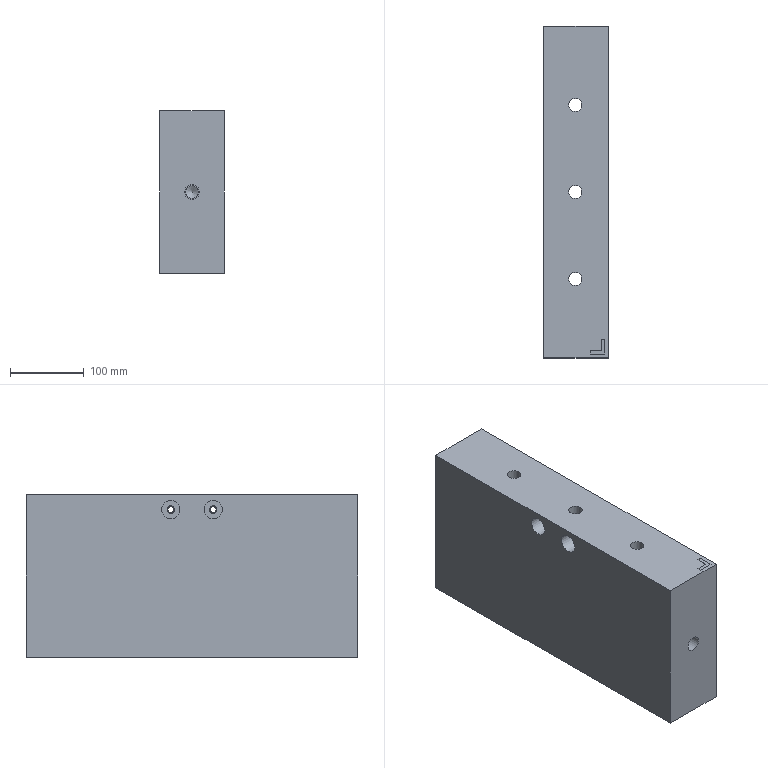Part | STEP file | CC01 | 1 solid | 108 faces | box 88 x 450 x 220 mm | volume 8457298 mm3 | plane 63 | other 18 | cylinder 15 | cone 12 | commonest cylinder face diameters 25 x4 18 x3 8 x2 12 x2 17.4 x2 20 x2